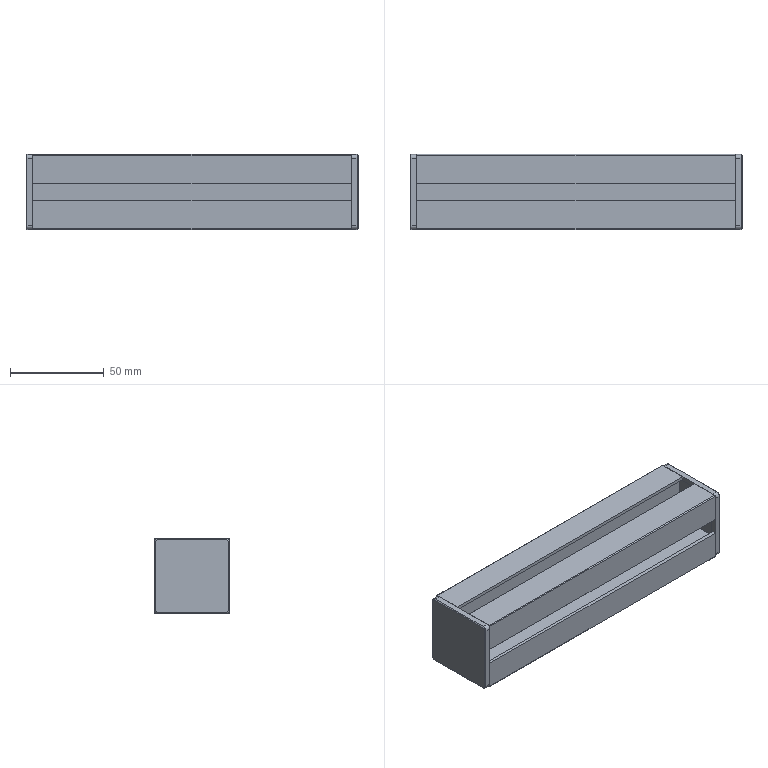Part | 3 solids | 323 faces | box 177 x 40 x 40 mm | volume 76492 mm3 | plane 220 | cylinder 55 | cone 48 | commonest cylinder face diameters 1.5 x32 4 x8 2.2 x6 14 x5 1 x4